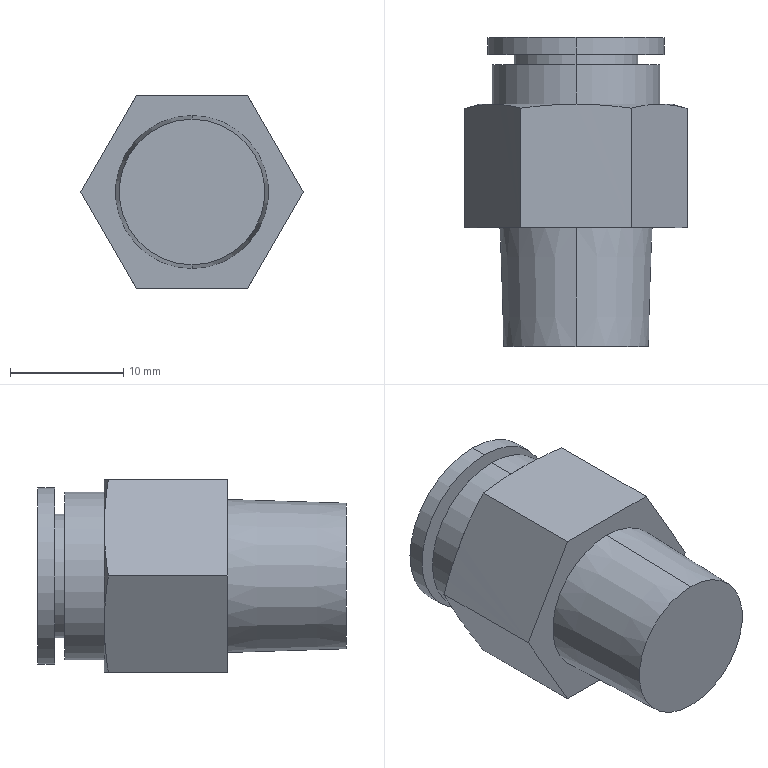Part | SolidWorks | features BaseBody 1 | 1 solid | 29 faces | box 19.63 x 27.3 x 17 mm | volume 3909 mm3 | plane 13 | cylinder 8 | cone 8 | commonest cylinder face diameters 10 x2 10.95 x2 14.8 x2 15.6 x2
STEP:
#1=CARTESIAN_POINT('',(0.,0.0226,-0.005));
#2=VERTEX_POINT('',#1);
#3=CARTESIAN_POINT('',(-0.000000001,0.0226,0.005));
#4=VERTEX_POINT('',#3);
#5=CARTESIAN_POINT('',(0.,0.0226,0.));
#6=DIRECTION('',(0.,-1.,0.));
#7=DIRECTION('',(-0.000000142,0.,1.));
#8=AXIS2_PLACEMENT_3D('',#5,#6,#7);
#9=CIRCLE('',#8,0.005);
#10=EDGE_CURVE('',#2,#4,#9,.T.);
#11=ORIENTED_EDGE('',*,*,#10,.F.);
#12=CARTESIAN_POINT('',(0.,0.007,-0.005));
#13=VERTEX_POINT('',#12);
#14=CARTESIAN_POINT('',(0.,0.007,-0.005));
#15=DIRECTION('',(0.,-1.,0.));
#16=VECTOR('',#15,1.);
#17=LINE('',#14,#16);
#18=EDGE_CURVE('',#2,#13,#17,.T.);
#19=ORIENTED_EDGE('',*,*,#18,.T.);
#20=CARTESIAN_POINT('',(0.,0.007,0.005));
#21=VERTEX_POINT('',#20);
#22=CARTESIAN_POINT('',(0.,0.007,0.));
#23=DIRECTION('',(0.,-1.,0.));
#24=DIRECTION('',(0.,0.,-1.));
#25=AXIS2_PLACEMENT_3D('',#22,#23,#24);
#26=CIRCLE('',#25,0.005);
#27=EDGE_CURVE('',#13,#21,#26,.T.);
#28=ORIENTED_EDGE('',*,*,#27,.T.);
#29=CARTESIAN_POINT('',(0.,0.007,0.005));
#30=DIRECTION('',(0.,-1.,0.));
#31=VECTOR('',#30,1.);
#32=LINE('',#29,#31);
#33=EDGE_CURVE('',#4,#21,#32,.T.);
#34=ORIENTED_EDGE('',*,*,#33,.F.);
#35=EDGE_LOOP('',(#11,#19,#28,#34));
#36=FACE_OUTER_BOUND('',#35,.T.);
#37=CARTESIAN_POINT('',(0.,0.007,0.));
#38=DIRECTION('',(0.,-1.,0.));
#39=DIRECTION('',(0.,0.,1.));
#40=AXIS2_PLACEMENT_3D('',#37,#38,#39);
#41=CYLINDRICAL_SURFACE('',#40,0.005);
#42=ADVANCED_FACE('',(#36),#41,.F.);
#43=CARTESIAN_POINT('',(0.,0.0202,0.0074));
#44=VERTEX_POINT('',#43);
#45=CARTESIAN_POINT('',(0.,0.0202,-0.0074));
#46=VERTEX_POINT('',#45);
#47=CARTESIAN_POINT('',(0.,0.0202,0.));
#48=DIRECTION('',(0.,-1.,0.));
#49=DIRECTION('',(0.,0.,-1.));
#50=AXIS2_PLACEMENT_3D('',#47,#48,#49);
#51=CIRCLE('',#50,0.0074);
#52=EDGE_CURVE('',#44,#46,#51,.T.);
#53=ORIENTED_EDGE('',*,*,#52,.T.);
#54=CARTESIAN_POINT('',(0.,0.0167,-0.0074));
#55=VERTEX_POINT('',#54);
#56=CARTESIAN_POINT('',(0.,-0.00601,-0.0074));
#57=DIRECTION('',(0.,-1.,0.));
#58=VECTOR('',#57,1.);
#59=LINE('',#56,#58);
#60=EDGE_CURVE('',#46,#55,#59,.T.);
#61=ORIENTED_EDGE('',*,*,#60,.T.);
#62=CARTESIAN_POINT('',(0.,0.0167,0.0074));
#63=VERTEX_POINT('',#62);
#64=CARTESIAN_POINT('',(0.,0.0167,0.));
#65=DIRECTION('',(0.,-1.,0.));
#66=DIRECTION('',(0.,0.,1.));
#67=AXIS2_PLACEMENT_3D('',#64,#65,#66);
#68=CIRCLE('',#67,0.0074);
#69=EDGE_CURVE('',#63,#55,#68,.T.);
#70=ORIENTED_EDGE('',*,*,#69,.F.);
#71=CARTESIAN_POINT('',(0.,-0.00601,0.0074));
#72=DIRECTION('',(0.,-1.,0.));
#73=VECTOR('',#72,1.);
#74=LINE('',#71,#73);
#75=EDGE_CURVE('',#44,#63,#74,.T.);
#76=ORIENTED_EDGE('',*,*,#75,.F.);
#77=EDGE_LOOP('',(#53,#61,#70,#76));
#78=FACE_OUTER_BOUND('',#77,.T.);
#79=CARTESIAN_POINT('',(0.,-0.00601,0.));
#80=DIRECTION('',(0.,-1.,0.));
#81=DIRECTION('',(0.,0.,1.));
#82=AXIS2_PLACEMENT_3D('',#79,#80,#81);
#83=CYLINDRICAL_SURFACE('',#82,0.0074);
#84=ADVANCED_FACE('',(#78),#83,.T.);
#85=CARTESIAN_POINT('',(0.,0.0211,0.005475));
#86=VERTEX_POINT('',#85);
#87=CARTESIAN_POINT('',(0.,0.0211,-0.005475));
#88=VERTEX_POINT('',#87);
#89=CARTESIAN_POINT('',(0.,0.0211,0.));
#90=DIRECTION('',(0.,-1.,0.));
#91=DIRECTION('',(0.,0.,-1.));
#92=AXIS2_PLACEMENT_3D('',#89,#90,#91);
#93=CIRCLE('',#92,0.005475);
#94=EDGE_CURVE('',#86,#88,#93,.T.);
#95=ORIENTED_EDGE('',*,*,#94,.T.);
#96=CARTESIAN_POINT('',(0.,0.0202,-0.005475));
#97=VERTEX_POINT('',#96);
#98=CARTESIAN_POINT('',(0.,-0.00601,-0.005475));
#99=DIRECTION('',(0.,-1.,0.));
#100=VECTOR('',#99,1.);
#101=LINE('',#98,#100);
#102=EDGE_CURVE('',#88,#97,#101,.T.);
#103=ORIENTED_EDGE('',*,*,#102,.T.);
#104=CARTESIAN_POINT('',(0.,0.0202,0.005475));
#105=VERTEX_POINT('',#104);
#106=CARTESIAN_POINT('',(0.,0.0202,0.));
#107=DIRECTION('',(0.,-1.,0.));
#108=DIRECTION('',(0.,0.,1.));
#109=AXIS2_PLACEMENT_3D('',#106,#107,#108);
#110=CIRCLE('',#109,0.005475);
#111=EDGE_CURVE('',#105,#97,#110,.T.);
#112=ORIENTED_EDGE('',*,*,#111,.F.);
#113=CARTESIAN_POINT('',(0.,-0.00601,0.005475));
#114=DIRECTION('',(0.,-1.,0.));
#115=VECTOR('',#114,1.);
#116=LINE('',#113,#115);
#117=EDGE_CURVE('',#86,#105,#116,.T.);
#118=ORIENTED_EDGE('',*,*,#117,.F.);
#119=EDGE_LOOP('',(#95,#103,#112,#118));
#120=FACE_OUTER_BOUND('',#119,.T.);
#121=CARTESIAN_POINT('',(0.,-0.00601,0.));
#122=DIRECTION('',(0.,-1.,0.));
#123=DIRECTION('',(0.000000001,0.,1.));
#124=AXIS2_PLACEMENT_3D('',#121,#122,#123);
#125=CYLINDRICAL_SURFACE('',#124,0.005475);
#126=ADVANCED_FACE('',(#120),#125,.T.);
#127=CARTESIAN_POINT('',(0.,0.0226,0.0078));
#128=VERTEX_POINT('',#127);
#129=CARTESIAN_POINT('',(0.,0.0226,-0.0078));
#130=VERTEX_POINT('',#129);
#131=CARTESIAN_POINT('',(0.,0.0226,0.));
#132=DIRECTION('',(0.,-1.,0.));
#133=DIRECTION('',(0.,0.,-1.));
#134=AXIS2_PLACEMENT_3D('',#131,#132,#133);
#135=CIRCLE('',#134,0.0078);
#136=EDGE_CURVE('',#128,#130,#135,.T.);
#137=ORIENTED_EDGE('',*,*,#136,.T.);
#138=CARTESIAN_POINT('',(0.,0.0211,-0.0078));
#139=VERTEX_POINT('',#138);
#140=CARTESIAN_POINT('',(0.,-0.00601,-0.0078));
#141=DIRECTION('',(0.,-1.,0.));
#142=VECTOR('',#141,1.);
#143=LINE('',#140,#142);
#144=EDGE_CURVE('',#130,#139,#143,.T.);
#145=ORIENTED_EDGE('',*,*,#144,.T.);
#146=CARTESIAN_POINT('',(0.,0.0211,0.0078));
#147=VERTEX_POINT('',#146);
#148=CARTESIAN_POINT('',(0.,0.0211,0.));
#149=DIRECTION('',(0.,-1.,0.));
#150=DIRECTION('',(0.,0.,1.));
#151=AXIS2_PLACEMENT_3D('',#148,#149,#150);
#152=CIRCLE('',#151,0.0078);
#153=EDGE_CURVE('',#147,#139,#152,.T.);
#154=ORIENTED_EDGE('',*,*,#153,.F.);
#155=CARTESIAN_POINT('',(0.,-0.00601,0.0078));
#156=DIRECTION('',(0.,-1.,0.));
#157=VECTOR('',#156,1.);
#158=LINE('',#155,#157);
#159=EDGE_CURVE('',#128,#147,#158,.T.);
#160=ORIENTED_EDGE('',*,*,#159,.F.);
#161=EDGE_LOOP('',(#137,#145,#154,#160));
#162=FACE_OUTER_BOUND('',#161,.T.);
#163=CARTESIAN_POINT('',(0.,-0.00601,0.));
#164=DIRECTION('',(0.,-1.,0.));
#165=DIRECTION('',(0.,0.,1.));
#166=AXIS2_PLACEMENT_3D('',#163,#164,#165);
#167=CYLINDRICAL_SURFACE('',#166,0.0078);
#168=ADVANCED_FACE('',(#162),#167,.T.);
#169=CARTESIAN_POINT('',(0.,-0.0047,0.006432));
#170=VERTEX_POINT('',#169);
#171=CARTESIAN_POINT('',(0.,-0.0047,-0.006432));
#172=VERTEX_POINT('',#171);
#173=CARTESIAN_POINT('',(0.,-0.0047,0.));
#174=DIRECTION('',(0.,-1.,0.));
#175=DIRECTION('',(0.,0.,1.));
#176=AXIS2_PLACEMENT_3D('',#173,#174,#175);
#177=CIRCLE('',#176,0.006432);
#178=EDGE_CURVE('',#170,#172,#177,.T.);
#179=ORIENTED_EDGE('',*,*,#178,.F.);
#180=CARTESIAN_POINT('',(0.,0.0058,0.00676));
#181=VERTEX_POINT('',#180);
#182=CARTESIAN_POINT('',(0.,0.0058,0.00676));
#183=DIRECTION('',(0.,0.9995,0.0312));
#184=VECTOR('',#183,1.);
#185=LINE('',#182,#184);
#186=EDGE_CURVE('',#170,#181,#185,.T.);
#187=ORIENTED_EDGE('',*,*,#186,.T.);
#188=CARTESIAN_POINT('',(0.,0.0058,-0.00676));
#189=VERTEX_POINT('',#188);
#190=CARTESIAN_POINT('',(0.,0.0058,0.));
#191=DIRECTION('',(0.,-1.,0.));
#192=DIRECTION('',(0.,0.,-1.));
#193=AXIS2_PLACEMENT_3D('',#190,#191,#192);
#194=CIRCLE('',#193,0.00676);
#195=EDGE_CURVE('',#181,#189,#194,.T.);
#196=ORIENTED_EDGE('',*,*,#195,.T.);
#197=CARTESIAN_POINT('',(0.,0.0058,-0.00676));
#198=DIRECTION('',(0.,0.9995,-0.0312));
#199=VECTOR('',#198,1.);
#200=LINE('',#197,#199);
#201=EDGE_CURVE('',#172,#189,#200,.T.);
#202=ORIENTED_EDGE('',*,*,#201,.F.);
#203=EDGE_LOOP('',(#179,#187,#196,#202));
#204=FACE_OUTER_BOUND('',#203,.T.);
#205=CARTESIAN_POINT('',(0.,0.0058,0.));
#206=DIRECTION('',(0.,1.,0.));
#207=DIRECTION('',(0.,0.,-1.));
#208=AXIS2_PLACEMENT_3D('',#205,#206,#207);
#209=CONICAL_SURFACE('',#208,0.00676,0.03121);
#210=ADVANCED_FACE('',(#204),#209,.T.);
#211=CARTESIAN_POINT('',(0.000000006,0.0167,-0.0085));
#212=VERTEX_POINT('',#211);
#213=CARTESIAN_POINT('',(0.007361,0.0167,-0.00425));
#214=VERTEX_POINT('',#213);
#215=CARTESIAN_POINT('',(0.,0.0167,0.));
#216=DIRECTION('',(0.,-1.,0.));
#217=DIRECTION('',(0.000000722,0.,-1.));
#218=AXIS2_PLACEMENT_3D('',#215,#216,#217);
#219=CIRCLE('',#218,0.0085);
#220=EDGE_CURVE('',#212,#214,#219,.T.);
#221=ORIENTED_EDGE('',*,*,#220,.T.);
#222=CARTESIAN_POINT('',(0.004907,0.01635,-0.0085));
#223=VERTEX_POINT('',#222);
#224=CARTESIAN_POINT('',(0.007361,0.0167,-0.00425));
#225=CARTESIAN_POINT('',(0.00715,0.0167,-0.004616));
#226=CARTESIAN_POINT('',(0.006938,0.01669,-0.004982));
#227=CARTESIAN_POINT('',(0.006614,0.01667,-0.005543));
#228=CARTESIAN_POINT('',(0.006505,0.01666,-0.005733));
#229=CARTESIAN_POINT('',(0.006293,0.01663,-0.0061));
#230=CARTESIAN_POINT('',(0.006189,0.01662,-0.00628));
#231=CARTESIAN_POINT('',(0.005988,0.01658,-0.006628));
#232=CARTESIAN_POINT('',(0.005891,0.01657,-0.006796));
#233=CARTESIAN_POINT('',(0.005699,0.01653,-0.007128));
#234=CARTESIAN_POINT('',(0.005603,0.01651,-0.007294));
#235=CARTESIAN_POINT('',(0.005313,0.01645,-0.007796));
#236=CARTESIAN_POINT('',(0.005118,0.0164,-0.008136));
#237=CARTESIAN_POINT('',(0.004907,0.01635,-0.0085));
#238=B_SPLINE_CURVE_WITH_KNOTS('',3,(#224,#225,#226,#227,#228,#229,#230,#231,#232,#233,#234,#235,#236,#237),.UNSPECIFIED.,.F.,.F.,(4,2,2,2,2,2,4),(0.,0.25,0.375,0.5,0.625,0.75,1.),.UNSPECIFIED.);
#239=EDGE_CURVE('',#214,#223,#238,.T.);
#240=ORIENTED_EDGE('',*,*,#239,.T.);
#241=CARTESIAN_POINT('',(0.004907,0.01635,-0.0085));
#242=CARTESIAN_POINT('',(0.004485,0.0164,-0.0085));
#243=CARTESIAN_POINT('',(0.004091,0.01645,-0.008499));
#244=CARTESIAN_POINT('',(0.003317,0.01653,-0.008499));
#245=CARTESIAN_POINT('',(0.002936,0.01657,-0.0085));
#246=CARTESIAN_POINT('',(0.002142,0.01663,-0.0085));
#247=CARTESIAN_POINT('',(0.001729,0.01666,-0.008499));
#248=CARTESIAN_POINT('',(0.0008548,0.01669,-0.008499));
#249=CARTESIAN_POINT('',(0.0004276,0.0167,-0.0085));
#250=CARTESIAN_POINT('',(0.000000006,0.0167,-0.0085));
#251=B_SPLINE_CURVE_WITH_KNOTS('',3,(#241,#242,#243,#244,#245,#246,#247,#248,#249,#250),.UNSPECIFIED.,.F.,.F.,(4,2,2,2,4),(0.,0.25,0.5,0.75,1.),.UNSPECIFIED.);
#252=EDGE_CURVE('',#223,#212,#251,.T.);
#253=ORIENTED_EDGE('',*,*,#252,.T.);
#254=EDGE_LOOP('',(#221,#240,#253));
#255=FACE_OUTER_BOUND('',#254,.T.);
#256=CARTESIAN_POINT('',(0.,0.01635,0.));
#257=DIRECTION('',(0.,-1.,0.));
#258=DIRECTION('',(0.000000722,0.,-1.));
#259=AXIS2_PLACEMENT_3D('',#256,#257,#258);
#260=CONICAL_SURFACE('',#259,0.009815,1.309);
#261=ADVANCED_FACE('',(#255),#260,.T.);
#262=CARTESIAN_POINT('',(0.007361,0.0167,0.00425));
#263=VERTEX_POINT('',#262);
#264=CARTESIAN_POINT('',(0.,0.0167,0.));
#265=DIRECTION('',(0.,-1.,0.));
#266=DIRECTION('',(0.866,0.,-0.5));
#267=AXIS2_PLACEMENT_3D('',#264,#265,#266);
#268=CIRCLE('',#267,0.0085);
#269=EDGE_CURVE('',#214,#263,#268,.T.);
#270=ORIENTED_EDGE('',*,*,#269,.T.);
#271=CARTESIAN_POINT('',(0.009815,0.01635,0.));
#272=VERTEX_POINT('',#271);
#273=CARTESIAN_POINT('',(0.007361,0.0167,0.00425));
#274=CARTESIAN_POINT('',(0.007573,0.0167,0.003884));
#275=CARTESIAN_POINT('',(0.007783,0.01669,0.003517));
#276=CARTESIAN_POINT('',(0.008107,0.01667,0.002956));
#277=CARTESIAN_POINT('',(0.008217,0.01666,0.002767));
#278=CARTESIAN_POINT('',(0.008429,0.01663,0.0024));
#279=CARTESIAN_POINT('',(0.008533,0.01662,0.00222));
#280=CARTESIAN_POINT('',(0.008734,0.01658,0.001871));
#281=CARTESIAN_POINT('',(0.008831,0.01657,0.001704));
#282=CARTESIAN_POINT('',(0.009022,0.01653,0.001371));
#283=CARTESIAN_POINT('',(0.009118,0.01651,0.001205));
#284=CARTESIAN_POINT('',(0.009408,0.01645,0.0007036));
#285=CARTESIAN_POINT('',(0.009605,0.0164,0.000364));
#286=CARTESIAN_POINT('',(0.009815,0.01635,0.));
#287=B_SPLINE_CURVE_WITH_KNOTS('',3,(#273,#274,#275,#276,#277,#278,#279,#280,#281,#282,#283,#284,#285,#286),.UNSPECIFIED.,.F.,.F.,(4,2,2,2,2,2,4),(0.,0.25,0.375,0.5,0.625,0.75,1.),.UNSPECIFIED.);
#288=EDGE_CURVE('',#263,#272,#287,.T.);
#289=ORIENTED_EDGE('',*,*,#288,.T.);
#290=CARTESIAN_POINT('',(0.009815,0.01635,0.));
#291=CARTESIAN_POINT('',(0.009604,0.0164,-0.0003661));
#292=CARTESIAN_POINT('',(0.009406,0.01645,-0.0007064));
#293=CARTESIAN_POINT('',(0.009019,0.01653,-0.001377));
#294=CARTESIAN_POINT('',(0.008829,0.01657,-0.001708));
#295=CARTESIAN_POINT('',(0.008432,0.01663,-0.002395));
#296=CARTESIAN_POINT('',(0.008225,0.01666,-0.002752));
#297=CARTESIAN_POINT('',(0.007788,0.01669,-0.003509));
#298=CARTESIAN_POINT('',(0.007575,0.0167,-0.003879));
#299=CARTESIAN_POINT('',(0.007361,0.0167,-0.00425));
#300=B_SPLINE_CURVE_WITH_KNOTS('',3,(#290,#291,#292,#293,#294,#295,#296,#297,#298,#299),.UNSPECIFIED.,.F.,.F.,(4,2,2,2,4),(0.,0.25,0.5,0.75,1.),.UNSPECIFIED.);
#301=EDGE_CURVE('',#272,#214,#300,.T.);
#302=ORIENTED_EDGE('',*,*,#301,.T.);
#303=EDGE_LOOP('',(#270,#289,#302));
#304=FACE_OUTER_BOUND('',#303,.T.);
#305=CARTESIAN_POINT('',(0.,0.01635,0.));
#306=DIRECTION('',(0.,-1.,0.));
#307=DIRECTION('',(0.866,0.,-0.5));
#308=AXIS2_PLACEMENT_3D('',#305,#306,#307);
#309=CONICAL_SURFACE('',#308,0.009815,1.309);
#310=ADVANCED_FACE('',(#304),#309,.T.);
#311=CARTESIAN_POINT('',(-0.007361,0.0167,-0.00425));
#312=VERTEX_POINT('',#311);
#313=CARTESIAN_POINT('',(0.,0.0167,0.));
#314=DIRECTION('',(0.,-1.,0.));
#315=DIRECTION('',(-0.866,0.,-0.5));
#316=AXIS2_PLACEMENT_3D('',#313,#314,#315);
#317=CIRCLE('',#316,0.0085);
#318=EDGE_CURVE('',#312,#212,#317,.T.);
#319=ORIENTED_EDGE('',*,*,#318,.T.);
#320=CARTESIAN_POINT('',(-0.004907,0.01635,-0.0085));
#321=VERTEX_POINT('',#320);
#322=CARTESIAN_POINT('',(0.000000006,0.0167,-0.0085));
#323=CARTESIAN_POINT('',(-0.0004189,0.0167,-0.0085));
#324=CARTESIAN_POINT('',(-0.0008374,0.01669,-0.008499));
#325=CARTESIAN_POINT('',(-0.001479,0.01667,-0.008499));
#326=CARTESIAN_POINT('',(-0.001696,0.01666,-0.008499));
#327=CARTESIAN_POINT('',(-0.002118,0.01663,-0.0085));
#328=CARTESIAN_POINT('',(-0.002325,0.01662,-0.0085));
#329=CARTESIAN_POINT('',(-0.002931,0.01657,-0.0085));
#330=CARTESIAN_POINT('',(-0.003307,0.01654,-0.008499));
#331=CARTESIAN_POINT('',(-0.004086,0.01645,-0.008499));
#332=CARTESIAN_POINT('',(-0.004483,0.0164,-0.0085));
#333=CARTESIAN_POINT('',(-0.004907,0.01635,-0.0085));
#334=B_SPLINE_CURVE_WITH_KNOTS('',3,(#322,#323,#324,#325,#326,#327,#328,#329,#330,#331,#332,#333),.UNSPECIFIED.,.F.,.F.,(4,2,2,2,2,4),(0.,0.25,0.375,0.5,0.75,1.),.UNSPECIFIED.);
#335=EDGE_CURVE('',#212,#321,#334,.T.);
#336=ORIENTED_EDGE('',*,*,#335,.T.);
#337=CARTESIAN_POINT('',(-0.004907,0.01635,-0.0085));
#338=CARTESIAN_POINT('',(-0.005119,0.0164,-0.008134));
#339=CARTESIAN_POINT('',(-0.005315,0.01645,-0.007793));
#340=CARTESIAN_POINT('',(-0.005702,0.01653,-0.007122));
#341=CARTESIAN_POINT('',(-0.005893,0.01657,-0.006792));
#342=CARTESIAN_POINT('',(-0.00629,0.01663,-0.006105));
#343=CARTESIAN_POINT('',(-0.006496,0.01666,-0.005748));
#344=CARTESIAN_POINT('',(-0.006933,0.01669,-0.00499));
#345=CARTESIAN_POINT('',(-0.007147,0.0167,-0.004621));
#346=CARTESIAN_POINT('',(-0.007361,0.0167,-0.00425));
#347=B_SPLINE_CURVE_WITH_KNOTS('',3,(#337,#338,#339,#340,#341,#342,#343,#344,#345,#346),.UNSPECIFIED.,.F.,.F.,(4,2,2,2,4),(0.,0.25,0.5,0.75,1.),.UNSPECIFIED.);
#348=EDGE_CURVE('',#321,#312,#347,.T.);
#349=ORIENTED_EDGE('',*,*,#348,.T.);
#350=EDGE_LOOP('',(#319,#336,#349));
#351=FACE_OUTER_BOUND('',#350,.T.);
#352=CARTESIAN_POINT('',(0.,0.01635,0.));
#353=DIRECTION('',(0.,-1.,0.));
#354=DIRECTION('',(-0.866,0.,-0.5));
#355=AXIS2_PLACEMENT_3D('',#352,#353,#354);
#356=CONICAL_SURFACE('',#355,0.009815,1.309);
#357=ADVANCED_FACE('',(#351),#356,.T.);
#358=CARTESIAN_POINT('',(-0.000000002,0.0167,0.0085));
#359=VERTEX_POINT('',#358);
#360=CARTESIAN_POINT('',(0.004907,0.01635,0.0085));
#361=VERTEX_POINT('',#360);
#362=CARTESIAN_POINT('',(-0.000000002,0.0167,0.0085));
#363=CARTESIAN_POINT('',(0.0004189,0.0167,0.0085));
#364=CARTESIAN_POINT('',(0.0008374,0.01669,0.008499));
#365=CARTESIAN_POINT('',(0.001479,0.01667,0.008499));
#366=CARTESIAN_POINT('',(0.001696,0.01666,0.008499));
#367=CARTESIAN_POINT('',(0.002118,0.01663,0.0085));
#368=CARTESIAN_POINT('',(0.002325,0.01662,0.0085));
#369=CARTESIAN_POINT('',(0.002931,0.01657,0.0085));
#370=CARTESIAN_POINT('',(0.003307,0.01654,0.008499));
#371=CARTESIAN_POINT('',(0.004086,0.01645,0.008499));
#372=CARTESIAN_POINT('',(0.004483,0.0164,0.0085));
#373=CARTESIAN_POINT('',(0.004907,0.01635,0.0085));
#374=B_SPLINE_CURVE_WITH_KNOTS('',3,(#362,#363,#364,#365,#366,#367,#368,#369,#370,#371,#372,#373),.UNSPECIFIED.,.F.,.F.,(4,2,2,2,2,4),(0.,0.25,0.375,0.5,0.75,1.),.UNSPECIFIED.);
#375=EDGE_CURVE('',#359,#361,#374,.T.);
#376=ORIENTED_EDGE('',*,*,#375,.T.);
#377=CARTESIAN_POINT('',(0.004907,0.01635,0.0085));
#378=CARTESIAN_POINT('',(0.005119,0.0164,0.008134));
#379=CARTESIAN_POINT('',(0.005315,0.01645,0.007793));
#380=CARTESIAN_POINT('',(0.005702,0.01653,0.007122));
#381=CARTESIAN_POINT('',(0.005893,0.01657,0.006792));
#382=CARTESIAN_POINT('',(0.00629,0.01663,0.006105));
#383=CARTESIAN_POINT('',(0.006496,0.01666,0.005748));
#384=CARTESIAN_POINT('',(0.006933,0.01669,0.00499));
#385=CARTESIAN_POINT('',(0.007147,0.0167,0.004621));
#386=CARTESIAN_POINT('',(0.007361,0.0167,0.00425));
#387=B_SPLINE_CURVE_WITH_KNOTS('',3,(#377,#378,#379,#380,#381,#382,#383,#384,#385,#386),.UNSPECIFIED.,.F.,.F.,(4,2,2,2,4),(0.,0.25,0.5,0.75,1.),.UNSPECIFIED.);
#388=EDGE_CURVE('',#361,#263,#387,.T.);
#389=ORIENTED_EDGE('',*,*,#388,.T.);
#390=CARTESIAN_POINT('',(0.,0.0167,0.));
#391=DIRECTION('',(0.,-1.,0.));
#392=DIRECTION('',(0.866,0.,0.5));
#393=AXIS2_PLACEMENT_3D('',#390,#391,#392);
#394=CIRCLE('',#393,0.0085);
#395=EDGE_CURVE('',#263,#359,#394,.T.);
#396=ORIENTED_EDGE('',*,*,#395,.T.);
#397=EDGE_LOOP('',(#376,#389,#396));
#398=FACE_OUTER_BOUND('',#397,.T.);
#399=CARTESIAN_POINT('',(0.,0.01635,0.));
#400=DIRECTION('',(0.,-1.,0.));
#401=DIRECTION('',(0.866,0.,0.5));
#402=AXIS2_PLACEMENT_3D('',#399,#400,#401);
#403=CONICAL_SURFACE('',#402,0.009815,1.309);
#404=ADVANCED_FACE('',(#398),#403,.T.);
#405=CARTESIAN_POINT('',(-0.007361,0.0167,0.00425));
#406=VERTEX_POINT('',#405);
#407=CARTESIAN_POINT('',(0.,0.0167,0.));
#408=DIRECTION('',(0.,-1.,0.));
#409=DIRECTION('',(-0.866,0.,0.5));
#410=AXIS2_PLACEMENT_3D('',#407,#408,#409);
#411=CIRCLE('',#410,0.0085);
#412=EDGE_CURVE('',#406,#312,#411,.T.);
#413=ORIENTED_EDGE('',*,*,#412,.T.);
#414=CARTESIAN_POINT('',(-0.009815,0.01635,0.));
#415=VERTEX_POINT('',#414);
#416=CARTESIAN_POINT('',(-0.007361,0.0167,-0.00425));
#417=CARTESIAN_POINT('',(-0.007573,0.0167,-0.003884));
#418=CARTESIAN_POINT('',(-0.007783,0.01669,-0.003517));
#419=CARTESIAN_POINT('',(-0.008107,0.01667,-0.002956));
#420=CARTESIAN_POINT('',(-0.008217,0.01666,-0.002767));
#421=CARTESIAN_POINT('',(-0.008429,0.01663,-0.0024));
#422=CARTESIAN_POINT('',(-0.008533,0.01662,-0.00222));
#423=CARTESIAN_POINT('',(-0.008734,0.01658,-0.001871));
#424=CARTESIAN_POINT('',(-0.008831,0.01657,-0.001704));
#425=CARTESIAN_POINT('',(-0.009022,0.01653,-0.001371));
#426=CARTESIAN_POINT('',(-0.009118,0.01651,-0.001205));
#427=CARTESIAN_POINT('',(-0.009408,0.01645,-0.0007036));
#428=CARTESIAN_POINT('',(-0.009605,0.0164,-0.000364));
#429=CARTESIAN_POINT('',(-0.009815,0.01635,0.));
#430=B_SPLINE_CURVE_WITH_KNOTS('',3,(#416,#417,#418,#419,#420,#421,#422,#423,#424,#425,#426,#427,#428,#429),.UNSPECIFIED.,.F.,.F.,(4,2,2,2,2,2,4),(0.,0.25,0.375,0.5,0.625,0.75,1.),.UNSPECIFIED.);
#431=EDGE_CURVE('',#312,#415,#430,.T.);
#432=ORIENTED_EDGE('',*,*,#431,.T.);
#433=CARTESIAN_POINT('',(-0.009815,0.01635,0.));
#434=CARTESIAN_POINT('',(-0.009604,0.0164,0.0003661));
#435=CARTESIAN_POINT('',(-0.009406,0.01645,0.0007064));
#436=CARTESIAN_POINT('',(-0.009019,0.01653,0.001377));
#437=CARTESIAN_POINT('',(-0.008829,0.01657,0.001708));
#438=CARTESIAN_POINT('',(-0.008432,0.01663,0.002395));
#439=CARTESIAN_POINT('',(-0.008225,0.01666,0.002752));
#440=CARTESIAN_POINT('',(-0.007788,0.01669,0.003509));
#441=CARTESIAN_POINT('',(-0.007575,0.0167,0.003879));
#442=CARTESIAN_POINT('',(-0.007361,0.0167,0.00425));
#443=B_SPLINE_CURVE_WITH_KNOTS('',3,(#433,#434,#435,#436,#437,#438,#439,#440,#441,#442),.UNSPECIFIED.,.F.,.F.,(4,2,2,2,4),(0.,0.25,0.5,0.75,1.),.UNSPECIFIED.);
#444=EDGE_CURVE('',#415,#406,#443,.T.);
#445=ORIENTED_EDGE('',*,*,#444,.T.);
#446=EDGE_LOOP('',(#413,#432,#445));
#447=FACE_OUTER_BOUND('',#446,.T.);
#448=CARTESIAN_POINT('',(0.,0.01635,0.));
#449=DIRECTION('',(0.,-1.,0.));
#450=DIRECTION('',(-0.866,0.,0.5));
#451=AXIS2_PLACEMENT_3D('',#448,#449,#450);
#452=CONICAL_SURFACE('',#451,0.009815,1.309);
#453=ADVANCED_FACE('',(#447),#452,.T.);
#454=ORIENTED_EDGE('',*,*,#136,.F.);
#455=CARTESIAN_POINT('',(0.,0.0226,0.));
#456=DIRECTION('',(0.,-1.,0.));
#457=DIRECTION('',(0.,0.,-1.));
#458=AXIS2_PLACEMENT_3D('',#455,#456,#457);
#459=CIRCLE('',#458,0.0078);
#460=EDGE_CURVE('',#130,#128,#459,.T.);
#461=ORIENTED_EDGE('',*,*,#460,.F.);
#462=EDGE_LOOP('',(#454,#461));
#463=FACE_OUTER_BOUND('',#462,.T.);
#464=CARTESIAN_POINT('',(0.,0.0226,0.));
#465=DIRECTION('',(0.,-1.,0.));
#466=DIRECTION('',(-0.000000142,0.,1.));
#467=AXIS2_PLACEMENT_3D('',#464,#465,#466);
#468=CIRCLE('',#467,0.005);
#469=EDGE_CURVE('',#4,#2,#468,.T.);
#470=ORIENTED_EDGE('',*,*,#469,.T.);
#471=ORIENTED_EDGE('',*,*,#10,.T.);
#472=EDGE_LOOP('',(#470,#471));
#473=FACE_BOUND('',#472,.T.);
#474=CARTESIAN_POINT('',(-0.008013,0.0226,0.0078));
#475=DIRECTION('',(0.,1.,0.));
#476=DIRECTION('',(1.,0.,0.));
#477=AXIS2_PLACEMENT_3D('',#474,#475,#476);
#478=PLANE('',#477);
#479=ADVANCED_FACE('',(#463,#473),#478,.T.);
#480=ORIENTED_EDGE('',*,*,#153,.T.);
#481=CARTESIAN_POINT('',(0.,0.0211,0.));
#482=DIRECTION('',(0.,-1.,0.));
#483=DIRECTION('',(0.,0.,1.));
#484=AXIS2_PLACEMENT_3D('',#481,#482,#483);
#485=CIRCLE('',#484,0.0078);
#486=EDGE_CURVE('',#139,#147,#485,.T.);
#487=ORIENTED_EDGE('',*,*,#486,.T.);
#488=EDGE_LOOP('',(#480,#487));
#489=FACE_OUTER_BOUND('',#488,.T.);
#490=ORIENTED_EDGE('',*,*,#94,.F.);
#491=CARTESIAN_POINT('',(0.,0.0211,0.));
#492=DIRECTION('',(0.,-1.,0.));
#493=DIRECTION('',(0.,0.,-1.));
#494=AXIS2_PLACEMENT_3D('',#491,#492,#493);
#495=CIRCLE('',#494,0.005475);
#496=EDGE_CURVE('',#88,#86,#495,.T.);
#497=ORIENTED_EDGE('',*,*,#496,.F.);
#498=EDGE_LOOP('',(#490,#497));
#499=FACE_BOUND('',#498,.T.);
#500=CARTESIAN_POINT('',(-0.008013,0.0211,-0.0078));
#501=DIRECTION('',(0.,-1.,0.));
#502=DIRECTION('',(1.,0.,0.));
#503=AXIS2_PLACEMENT_3D('',#500,#501,#502);
#504=PLANE('',#503);
#505=ADVANCED_FACE('',(#489,#499),#504,.T.);
#506=ORIENTED_EDGE('',*,*,#52,.F.);
#507=CARTESIAN_POINT('',(0.,0.0202,0.));
#508=DIRECTION('',(0.,-1.,0.));
#509=DIRECTION('',(0.,0.,-1.));
#510=AXIS2_PLACEMENT_3D('',#507,#508,#509);
#511=CIRCLE('',#510,0.0074);
#512=EDGE_CURVE('',#46,#44,#511,.T.);
#513=ORIENTED_EDGE('',*,*,#512,.F.);
#514=EDGE_LOOP('',(#506,#513));
#515=FACE_OUTER_BOUND('',#514,.T.);
#516=ORIENTED_EDGE('',*,*,#111,.T.);
#517=CARTESIAN_POINT('',(0.,0.0202,0.));
#518=DIRECTION('',(0.,-1.,0.));
#519=DIRECTION('',(0.,0.,1.));
#520=AXIS2_PLACEMENT_3D('',#517,#518,#519);
#521=CIRCLE('',#520,0.005475);
#522=EDGE_CURVE('',#97,#105,#521,.T.);
#523=ORIENTED_EDGE('',*,*,#522,.T.);
#524=EDGE_LOOP('',(#516,#523));
#525=FACE_BOUND('',#524,.T.);
#526=CARTESIAN_POINT('',(-0.007602,0.0202,0.0074));
#527=DIRECTION('',(0.,1.,0.));
#528=DIRECTION('',(1.,0.,0.));
#529=AXIS2_PLACEMENT_3D('',#526,#527,#528);
#530=PLANE('',#529);
#531=ADVANCED_FACE('',(#515,#525),#530,.T.);
#532=ORIENTED_EDGE('',*,*,#269,.F.);
#533=ORIENTED_EDGE('',*,*,#220,.F.);
#534=ORIENTED_EDGE('',*,*,#318,.F.);
#535=ORIENTED_EDGE('',*,*,#412,.F.);
#536=CARTESIAN_POINT('',(0.,0.0167,0.));
#537=DIRECTION('',(0.,-1.,0.));
#538=DIRECTION('',(-0.866,0.,0.5));
#539=AXIS2_PLACEMENT_3D('',#536,#537,#538);
#540=CIRCLE('',#539,0.0085);
#541=EDGE_CURVE('',#359,#406,#540,.T.);
#542=ORIENTED_EDGE('',*,*,#541,.F.);
#543=ORIENTED_EDGE('',*,*,#395,.F.);
#544=EDGE_LOOP('',(#532,#533,#534,#535,#542,#543));
#545=FACE_OUTER_BOUND('',#544,.T.);
#546=ORIENTED_EDGE('',*,*,#69,.T.);
#547=CARTESIAN_POINT('',(0.,0.0167,0.));
#548=DIRECTION('',(0.,-1.,0.));
#549=DIRECTION('',(0.,0.,1.));
#550=AXIS2_PLACEMENT_3D('',#547,#548,#549);
#551=CIRCLE('',#550,0.0074);
#552=EDGE_CURVE('',#55,#63,#551,.T.);
#553=ORIENTED_EDGE('',*,*,#552,.T.);
#554=EDGE_LOOP('',(#546,#553));
#555=FACE_BOUND('',#554,.T.);
#556=CARTESIAN_POINT('',(-0.0085,0.0167,0.0085));
#557=DIRECTION('',(0.,1.,0.));
#558=DIRECTION('',(1.,0.,0.));
#559=AXIS2_PLACEMENT_3D('',#556,#557,#558);
#560=PLANE('',#559);
#561=ADVANCED_FACE('',(#545,#555),#560,.T.);
#562=CARTESIAN_POINT('',(-0.004907,0.01635,0.0085));
#563=VERTEX_POINT('',#562);
#564=CARTESIAN_POINT('',(-0.007361,0.0167,0.00425));
#565=CARTESIAN_POINT('',(-0.00715,0.0167,0.004616));
#566=CARTESIAN_POINT('',(-0.006938,0.01669,0.004982));
#567=CARTESIAN_POINT('',(-0.006614,0.01667,0.005543));
#568=CARTESIAN_POINT('',(-0.006505,0.01666,0.005733));
#569=CARTESIAN_POINT('',(-0.006293,0.01663,0.0061));
#570=CARTESIAN_POINT('',(-0.006189,0.01662,0.00628));
#571=CARTESIAN_POINT('',(-0.005988,0.01658,0.006628));
#572=CARTESIAN_POINT('',(-0.005891,0.01657,0.006796));
#573=CARTESIAN_POINT('',(-0.005699,0.01653,0.007128));
#574=CARTESIAN_POINT('',(-0.005603,0.01651,0.007294));
#575=CARTESIAN_POINT('',(-0.005313,0.01645,0.007796));
#576=CARTESIAN_POINT('',(-0.005118,0.0164,0.008136));
#577=CARTESIAN_POINT('',(-0.004907,0.01635,0.0085));
#578=B_SPLINE_CURVE_WITH_KNOTS('',3,(#564,#565,#566,#567,#568,#569,#570,#571,#572,#573,#574,#575,#576,#577),.UNSPECIFIED.,.F.,.F.,(4,2,2,2,2,2,4),(0.,0.25,0.375,0.5,0.625,0.75,1.),.UNSPECIFIED.);
#579=EDGE_CURVE('',#406,#563,#578,.T.);
#580=ORIENTED_EDGE('',*,*,#579,.T.);
#581=CARTESIAN_POINT('',(-0.004907,0.01635,0.0085));
#582=CARTESIAN_POINT('',(-0.004485,0.0164,0.0085));
#583=CARTESIAN_POINT('',(-0.004091,0.01645,0.008499));
#584=CARTESIAN_POINT('',(-0.003317,0.01653,0.008499));
#585=CARTESIAN_POINT('',(-0.002936,0.01657,0.0085));
#586=CARTESIAN_POINT('',(-0.002142,0.01663,0.0085));
#587=CARTESIAN_POINT('',(-0.001729,0.01666,0.008499));
#588=CARTESIAN_POINT('',(-0.0008548,0.01669,0.008499));
#589=CARTESIAN_POINT('',(-0.0004276,0.0167,0.0085));
#590=CARTESIAN_POINT('',(-0.000000002,0.0167,0.0085));
#591=B_SPLINE_CURVE_WITH_KNOTS('',3,(#581,#582,#583,#584,#585,#586,#587,#588,#589,#590),.UNSPECIFIED.,.F.,.F.,(4,2,2,2,4),(0.,0.25,0.5,0.75,1.),.UNSPECIFIED.);
#592=EDGE_CURVE('',#563,#359,#591,.T.);
#593=ORIENTED_EDGE('',*,*,#592,.T.);
#594=ORIENTED_EDGE('',*,*,#541,.T.);
#595=EDGE_LOOP('',(#580,#593,#594));
#596=FACE_OUTER_BOUND('',#595,.T.);
#597=CARTESIAN_POINT('',(0.,0.01635,0.));
#598=DIRECTION('',(0.,-1.,0.));
#599=DIRECTION('',(-0.000000241,0.,1.));
#600=AXIS2_PLACEMENT_3D('',#597,#598,#599);
#601=CONICAL_SURFACE('',#600,0.009815,1.309);
#602=ADVANCED_FACE('',(#596),#601,.T.);
#603=CARTESIAN_POINT('',(-0.004907,0.0058,-0.0085));
#604=VERTEX_POINT('',#603);
#605=CARTESIAN_POINT('',(-0.004907,0.01635,-0.0085));
#606=DIRECTION('',(-0.000000001,-1.,0.000000002));
#607=VECTOR('',#606,1.);
#608=LINE('',#605,#607);
#609=EDGE_CURVE('',#321,#604,#608,.T.);
#610=ORIENTED_EDGE('',*,*,#609,.T.);
#611=CARTESIAN_POINT('',(-0.009815,0.0058,0.));
#612=VERTEX_POINT('',#611);
#613=CARTESIAN_POINT('',(-0.004907,0.0058,-0.0085));
#614=DIRECTION('',(0.5,0.,-0.866));
#615=VECTOR('',#614,1.);
#616=LINE('',#613,#615);
#617=EDGE_CURVE('',#612,#604,#616,.T.);
#618=ORIENTED_EDGE('',*,*,#617,.F.);
#619=CARTESIAN_POINT('',(-0.009815,0.0058,0.));
#620=DIRECTION('',(0.,-1.,0.));
#621=VECTOR('',#620,1.);
#622=LINE('',#619,#621);
#623=EDGE_CURVE('',#415,#612,#622,.T.);
#624=ORIENTED_EDGE('',*,*,#623,.F.);
#625=ORIENTED_EDGE('',*,*,#431,.F.);
#626=ORIENTED_EDGE('',*,*,#348,.F.);
#627=EDGE_LOOP('',(#610,#618,#624,#625,#626));
#628=FACE_OUTER_BOUND('',#627,.T.);
#629=CARTESIAN_POINT('',(-0.009815,0.0058,0.));
#630=DIRECTION('',(-0.866,0.,-0.5));
#631=DIRECTION('',(0.,1.,0.));
#632=AXIS2_PLACEMENT_3D('',#629,#630,#631);
#633=PLANE('',#632);
#634=ADVANCED_FACE('',(#628),#633,.T.);
#635=CARTESIAN_POINT('',(0.004907,0.0058,-0.0085));
#636=VERTEX_POINT('',#635);
#637=CARTESIAN_POINT('',(0.004907,0.01635,-0.0085));
#638=DIRECTION('',(0.,-1.,0.));
#639=VECTOR('',#638,1.);
#640=LINE('',#637,#639);
#641=EDGE_CURVE('',#223,#636,#640,.T.);
#642=ORIENTED_EDGE('',*,*,#641,.T.);
#643=CARTESIAN_POINT('',(0.004907,0.0058,-0.0085));
#644=DIRECTION('',(1.,0.,0.));
#645=VECTOR('',#644,1.);
#646=LINE('',#643,#645);
#647=EDGE_CURVE('',#604,#636,#646,.T.);
#648=ORIENTED_EDGE('',*,*,#647,.F.);
#649=ORIENTED_EDGE('',*,*,#609,.F.);
#650=ORIENTED_EDGE('',*,*,#335,.F.);
#651=ORIENTED_EDGE('',*,*,#252,.F.);
#652=EDGE_LOOP('',(#642,#648,#649,#650,#651));
#653=FACE_OUTER_BOUND('',#652,.T.);
#654=CARTESIAN_POINT('',(-0.004907,0.0058,-0.0085));
#655=DIRECTION('',(0.,0.,-1.));
#656=DIRECTION('',(0.,1.,0.));
#657=AXIS2_PLACEMENT_3D('',#654,#655,#656);
#658=PLANE('',#657);
#659=ADVANCED_FACE('',(#653),#658,.T.);
#660=CARTESIAN_POINT('',(0.009815,0.0058,0.));
#661=VERTEX_POINT('',#660);
#662=CARTESIAN_POINT('',(0.009815,0.01635,0.));
#663=DIRECTION('',(0.,-1.,0.));
#664=VECTOR('',#663,1.);
#665=LINE('',#662,#664);
#666=EDGE_CURVE('',#272,#661,#665,.T.);
#667=ORIENTED_EDGE('',*,*,#666,.T.);
#668=CARTESIAN_POINT('',(0.009815,0.0058,0.));
#669=DIRECTION('',(0.5,0.,0.866));
#670=VECTOR('',#669,1.);
#671=LINE('',#668,#670);
#672=EDGE_CURVE('',#636,#661,#671,.T.);
#673=ORIENTED_EDGE('',*,*,#672,.F.);
#674=ORIENTED_EDGE('',*,*,#641,.F.);
#675=ORIENTED_EDGE('',*,*,#239,.F.);
#676=ORIENTED_EDGE('',*,*,#301,.F.);
#677=EDGE_LOOP('',(#667,#673,#674,#675,#676));
#678=FACE_OUTER_BOUND('',#677,.T.);
#679=CARTESIAN_POINT('',(0.004907,0.0058,-0.0085));
#680=DIRECTION('',(0.866,0.,-0.5));
#681=DIRECTION('',(0.,1.,0.));
#682=AXIS2_PLACEMENT_3D('',#679,#680,#681);
#683=PLANE('',#682);
#684=ADVANCED_FACE('',(#678),#683,.T.);
#685=CARTESIAN_POINT('',(0.004907,0.0058,0.0085));
#686=VERTEX_POINT('',#685);
#687=CARTESIAN_POINT('',(0.004907,0.01635,0.0085));
#688=DIRECTION('',(0.000000001,-1.,-0.000000002));
#689=VECTOR('',#688,1.);
#690=LINE('',#687,#689);
#691=EDGE_CURVE('',#361,#686,#690,.T.);
#692=ORIENTED_EDGE('',*,*,#691,.T.);
#693=CARTESIAN_POINT('',(0.004907,0.0058,0.0085));
#694=DIRECTION('',(-0.5,0.,0.866));
#695=VECTOR('',#694,1.);
#696=LINE('',#693,#695);
#697=EDGE_CURVE('',#661,#686,#696,.T.);
#698=ORIENTED_EDGE('',*,*,#697,.F.);
#699=ORIENTED_EDGE('',*,*,#666,.F.);
#700=ORIENTED_EDGE('',*,*,#288,.F.);
#701=ORIENTED_EDGE('',*,*,#388,.F.);
#702=EDGE_LOOP('',(#692,#698,#699,#700,#701));
#703=FACE_OUTER_BOUND('',#702,.T.);
#704=CARTESIAN_POINT('',(0.009815,0.0058,0.));
#705=DIRECTION('',(0.866,0.,0.5));
#706=DIRECTION('',(0.,1.,0.));
#707=AXIS2_PLACEMENT_3D('',#704,#705,#706);
#708=PLANE('',#707);
#709=ADVANCED_FACE('',(#703),#708,.T.);
#710=CARTESIAN_POINT('',(-0.004907,0.0058,0.0085));
#711=VERTEX_POINT('',#710);
#712=CARTESIAN_POINT('',(-0.004907,0.01635,0.0085));
#713=DIRECTION('',(0.,-1.,0.));
#714=VECTOR('',#713,1.);
#715=LINE('',#712,#714);
#716=EDGE_CURVE('',#563,#711,#715,.T.);
#717=ORIENTED_EDGE('',*,*,#716,.T.);
#718=CARTESIAN_POINT('',(-0.004907,0.0058,0.0085));
#719=DIRECTION('',(-1.,0.,0.));
#720=VECTOR('',#719,1.);
#721=LINE('',#718,#720);
#722=EDGE_CURVE('',#686,#711,#721,.T.);
#723=ORIENTED_EDGE('',*,*,#722,.F.);
#724=ORIENTED_EDGE('',*,*,#691,.F.);
#725=ORIENTED_EDGE('',*,*,#375,.F.);
#726=ORIENTED_EDGE('',*,*,#592,.F.);
#727=EDGE_LOOP('',(#717,#723,#724,#725,#726));
#728=FACE_OUTER_BOUND('',#727,.T.);
#729=CARTESIAN_POINT('',(0.004907,0.0058,0.0085));
#730=DIRECTION('',(0.,0.,1.));
#731=DIRECTION('',(0.,1.,0.));
#732=AXIS2_PLACEMENT_3D('',#729,#730,#731);
#733=PLANE('',#732);
#734=ADVANCED_FACE('',(#728),#733,.T.);
#735=ORIENTED_EDGE('',*,*,#623,.T.);
#736=CARTESIAN_POINT('',(-0.009815,0.0058,0.));
#737=DIRECTION('',(-0.5,0.,-0.866));
#738=VECTOR('',#737,1.);
#739=LINE('',#736,#738);
#740=EDGE_CURVE('',#711,#612,#739,.T.);
#741=ORIENTED_EDGE('',*,*,#740,.F.);
#742=ORIENTED_EDGE('',*,*,#716,.F.);
#743=ORIENTED_EDGE('',*,*,#579,.F.);
#744=ORIENTED_EDGE('',*,*,#444,.F.);
#745=EDGE_LOOP('',(#735,#741,#742,#743,#744));
#746=FACE_OUTER_BOUND('',#745,.T.);
#747=CARTESIAN_POINT('',(-0.004907,0.0058,0.0085));
#748=DIRECTION('',(-0.866,0.,0.5));
#749=DIRECTION('',(0.,1.,0.));
#750=AXIS2_PLACEMENT_3D('',#747,#748,#749);
#751=PLANE('',#750);
#752=ADVANCED_FACE('',(#746),#751,.T.);
#753=ORIENTED_EDGE('',*,*,#740,.T.);
#754=ORIENTED_EDGE('',*,*,#617,.T.);
#755=ORIENTED_EDGE('',*,*,#647,.T.);
#756=ORIENTED_EDGE('',*,*,#672,.T.);
#757=ORIENTED_EDGE('',*,*,#697,.T.);
#758=ORIENTED_EDGE('',*,*,#722,.T.);
#759=EDGE_LOOP('',(#753,#754,#755,#756,#757,#758));
#760=FACE_OUTER_BOUND('',#759,.T.);
#761=CARTESIAN_POINT('',(0.,0.0058,0.));
#762=DIRECTION('',(0.,-1.,0.));
#763=DIRECTION('',(0.,0.,-1.));
#764=AXIS2_PLACEMENT_3D('',#761,#762,#763);
#765=CIRCLE('',#764,0.00676);
#766=EDGE_CURVE('',#189,#181,#765,.T.);
#767=ORIENTED_EDGE('',*,*,#766,.F.);
#768=ORIENTED_EDGE('',*,*,#195,.F.);
#769=EDGE_LOOP('',(#767,#768));
#770=FACE_BOUND('',#769,.T.);
#771=CARTESIAN_POINT('',(-0.009815,0.0058,-0.0085));
#772=DIRECTION('',(0.,-1.,0.));
#773=DIRECTION('',(1.,0.,0.));
#774=AXIS2_PLACEMENT_3D('',#771,#772,#773);
#775=PLANE('',#774);
#776=ADVANCED_FACE('',(#760,#770),#775,.T.);
#777=CARTESIAN_POINT('',(0.,0.007,0.));
#778=DIRECTION('',(0.,-1.,0.));
#779=DIRECTION('',(0.,0.,-1.));
#780=AXIS2_PLACEMENT_3D('',#777,#778,#779);
#781=CIRCLE('',#780,0.005);
#782=EDGE_CURVE('',#21,#13,#781,.T.);
#783=ORIENTED_EDGE('',*,*,#782,.F.);
#784=ORIENTED_EDGE('',*,*,#27,.F.);
#785=EDGE_LOOP('',(#783,#784));
#786=FACE_OUTER_BOUND('',#785,.T.);
#787=CARTESIAN_POINT('',(-0.005,0.007,-0.005));
#788=DIRECTION('',(0.,1.,0.));
#789=DIRECTION('',(0.,0.,1.));
#790=AXIS2_PLACEMENT_3D('',#787,#788,#789);
#791=PLANE('',#790);
#792=ADVANCED_FACE('',(#786),#791,.T.);
#793=CARTESIAN_POINT('',(0.,-0.0047,0.));
#794=DIRECTION('',(0.,-1.,0.));
#795=DIRECTION('',(0.,0.,1.));
#796=AXIS2_PLACEMENT_3D('',#793,#794,#795);
#797=CIRCLE('',#796,0.006432);
#798=EDGE_CURVE('',#172,#170,#797,.T.);
#799=ORIENTED_EDGE('',*,*,#798,.T.);
#800=ORIENTED_EDGE('',*,*,#178,.T.);
#801=EDGE_LOOP('',(#799,#800));
#802=FACE_OUTER_BOUND('',#801,.T.);
#803=CARTESIAN_POINT('',(-0.006608,-0.0047,0.006432));
#804=DIRECTION('',(0.,-1.,0.));
#805=DIRECTION('',(0.,0.,-1.));
#806=AXIS2_PLACEMENT_3D('',#803,#804,#805);
#807=PLANE('',#806);
#808=ADVANCED_FACE('',(#802),#807,.T.);
#809=ORIENTED_EDGE('',*,*,#186,.F.);
#810=ORIENTED_EDGE('',*,*,#798,.F.);
#811=ORIENTED_EDGE('',*,*,#201,.T.);
#812=ORIENTED_EDGE('',*,*,#766,.T.);
#813=EDGE_LOOP('',(#809,#810,#811,#812));
#814=FACE_OUTER_BOUND('',#813,.T.);
#815=CARTESIAN_POINT('',(0.,0.0058,0.));
#816=DIRECTION('',(0.,1.,0.));
#817=DIRECTION('',(0.,0.,-1.));
#818=AXIS2_PLACEMENT_3D('',#815,#816,#817);
#819=CONICAL_SURFACE('',#818,0.00676,0.03121);
#820=ADVANCED_FACE('',(#814),#819,.T.);
#821=ORIENTED_EDGE('',*,*,#144,.F.);
#822=ORIENTED_EDGE('',*,*,#460,.T.);
#823=ORIENTED_EDGE('',*,*,#159,.T.);
#824=ORIENTED_EDGE('',*,*,#486,.F.);
#825=EDGE_LOOP('',(#821,#822,#823,#824));
#826=FACE_OUTER_BOUND('',#825,.T.);
#827=CARTESIAN_POINT('',(0.,-0.00601,0.));
#828=DIRECTION('',(0.,-1.,0.));
#829=DIRECTION('',(0.,0.,1.));
#830=AXIS2_PLACEMENT_3D('',#827,#828,#829);
#831=CYLINDRICAL_SURFACE('',#830,0.0078);
#832=ADVANCED_FACE('',(#826),#831,.T.);
#833=ORIENTED_EDGE('',*,*,#102,.F.);
#834=ORIENTED_EDGE('',*,*,#496,.T.);
#835=ORIENTED_EDGE('',*,*,#117,.T.);
#836=ORIENTED_EDGE('',*,*,#522,.F.);
#837=EDGE_LOOP('',(#833,#834,#835,#836));
#838=FACE_OUTER_BOUND('',#837,.T.);
#839=CARTESIAN_POINT('',(0.,-0.00601,0.));
#840=DIRECTION('',(0.,-1.,0.));
#841=DIRECTION('',(0.000000001,0.,1.));
#842=AXIS2_PLACEMENT_3D('',#839,#840,#841);
#843=CYLINDRICAL_SURFACE('',#842,0.005475);
#844=ADVANCED_FACE('',(#838),#843,.T.);
#845=ORIENTED_EDGE('',*,*,#60,.F.);
#846=ORIENTED_EDGE('',*,*,#512,.T.);
#847=ORIENTED_EDGE('',*,*,#75,.T.);
#848=ORIENTED_EDGE('',*,*,#552,.F.);
#849=EDGE_LOOP('',(#845,#846,#847,#848));
#850=FACE_OUTER_BOUND('',#849,.T.);
#851=CARTESIAN_POINT('',(0.,-0.00601,0.));
#852=DIRECTION('',(0.,-1.,0.));
#853=DIRECTION('',(0.,0.,1.));
#854=AXIS2_PLACEMENT_3D('',#851,#852,#853);
#855=CYLINDRICAL_SURFACE('',#854,0.0074);
#856=ADVANCED_FACE('',(#850),#855,.T.);
#857=ORIENTED_EDGE('',*,*,#18,.F.);
#858=ORIENTED_EDGE('',*,*,#469,.F.);
#859=ORIENTED_EDGE('',*,*,#33,.T.);
#860=ORIENTED_EDGE('',*,*,#782,.T.);
#861=EDGE_LOOP('',(#857,#858,#859,#860));
#862=FACE_OUTER_BOUND('',#861,.T.);
#863=CARTESIAN_POINT('',(0.,0.007,0.));
#864=DIRECTION('',(0.,-1.,0.));
#865=DIRECTION('',(0.,0.,1.));
#866=AXIS2_PLACEMENT_3D('',#863,#864,#865);
#867=CYLINDRICAL_SURFACE('',#866,0.005);
#868=ADVANCED_FACE('',(#862),#867,.F.);
#869=CLOSED_SHELL('',(#42,#84,#126,#168,#210,#261,#310,#357,#404,#453,#479,#505,#531,#561,#602,#634,#659,#684,#709,#734,#752,#776,#792,#808,#820,#832,#844,#856,#868));
#870=MANIFOLD_SOLID_BREP('',#869);
#871=CARTESIAN_POINT('',(0.,0.,0.));
#872=DIRECTION('',(0.,0.,1.));
#873=DIRECTION('',(1.,0.,0.));
#874=AXIS2_PLACEMENT_3D('',#871,#872,#873);
#875=(LENGTH_UNIT()NAMED_UNIT(*)SI_UNIT($,.METRE.));
#876=UNCERTAINTY_MEASURE_WITH_UNIT(LENGTH_MEASURE(0.00001),#875,'','');
#877=(NAMED_UNIT(*)PLANE_ANGLE_UNIT()SI_UNIT($,.RADIAN.));
#878=(NAMED_UNIT(*)SI_UNIT($,.STERADIAN.)SOLID_ANGLE_UNIT());
#879=(GEOMETRIC_REPRESENTATION_CONTEXT(3)GLOBAL_UNCERTAINTY_ASSIGNED_CONTEXT((#876))GLOBAL_UNIT_ASSIGNED_CONTEXT((#875,#877,#878))REPRESENTATION_CONTEXT('',''));
#880=ADVANCED_BREP_SHAPE_REPRESENTATION('',(#870,#874),#879);